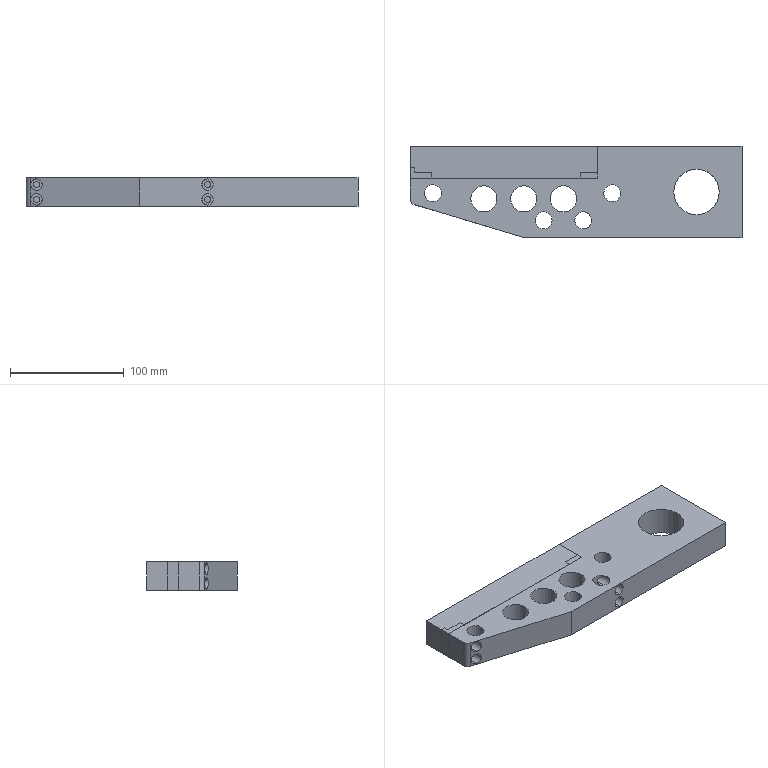Part | 2 solids | 84 faces | box 292 x 80 x 25 mm | volume 458763 mm3 | cylinder 47 | plane 25 | cone 12 | commonest cylinder face diameters 5.2 x12 10 x11 5.5 x8 15 x8 23 x6 40 x2